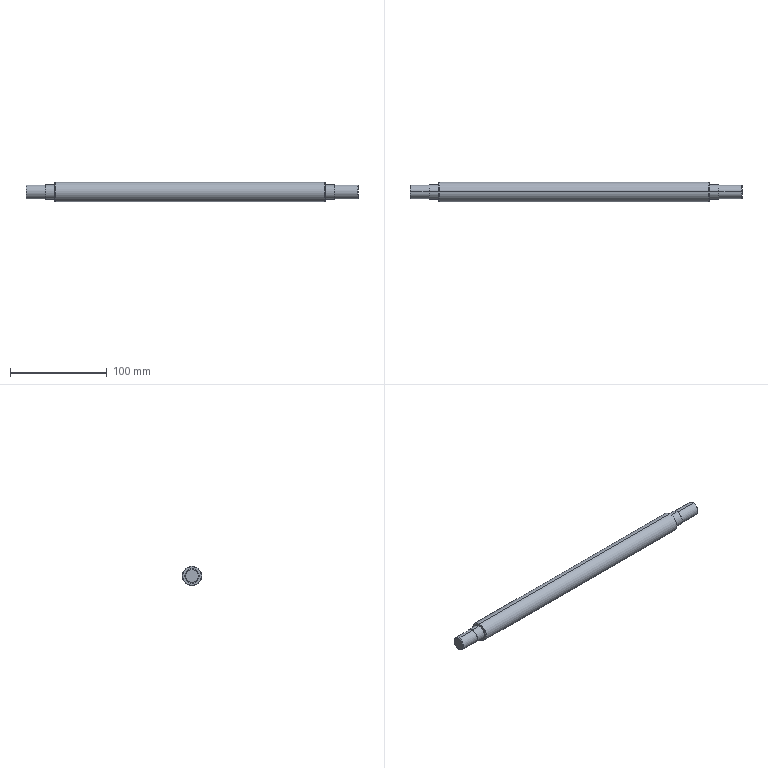Part | SolidWorks | features BaseBody 1 | 1 solid | 24 faces | box 344 x 20 x 20 mm | volume 98246 mm3 | cylinder 10 | cone 8 | plane 6 | commonest cylinder face diameters 14 x4 15 x4 20 x2
STEP:
#1=CARTESIAN_POINT('',(172.,0.,6.5));
#2=VERTEX_POINT('',#1);
#3=CARTESIAN_POINT('',(172.,0.,-6.5));
#4=VERTEX_POINT('',#3);
#5=CARTESIAN_POINT('',(172.,0.,0.));
#6=DIRECTION('',(-1.,0.,0.));
#7=DIRECTION('',(0.,0.,1.));
#8=AXIS2_PLACEMENT_3D('',#5,#6,#7);
#9=CIRCLE('',#8,6.5);
#10=EDGE_CURVE('',#2,#4,#9,.T.);
#11=ORIENTED_EDGE('',*,*,#10,.T.);
#12=CARTESIAN_POINT('',(171.5,0.,-7.));
#13=VERTEX_POINT('',#12);
#14=CARTESIAN_POINT('',(172.,0.,-6.5));
#15=DIRECTION('',(-0.7071,0.,-0.7071));
#16=VECTOR('',#15,1000.);
#17=LINE('',#14,#16);
#18=EDGE_CURVE('',#4,#13,#17,.T.);
#19=ORIENTED_EDGE('',*,*,#18,.T.);
#20=CARTESIAN_POINT('',(171.5,0.,7.));
#21=VERTEX_POINT('',#20);
#22=CARTESIAN_POINT('',(171.5,0.,0.));
#23=DIRECTION('',(-1.,0.,0.));
#24=DIRECTION('',(0.,0.,1.));
#25=AXIS2_PLACEMENT_3D('',#22,#23,#24);
#26=CIRCLE('',#25,7.);
#27=EDGE_CURVE('',#21,#13,#26,.T.);
#28=ORIENTED_EDGE('',*,*,#27,.F.);
#29=CARTESIAN_POINT('',(172.,0.,6.5));
#30=DIRECTION('',(-0.7071,0.,0.7071));
#31=VECTOR('',#30,1000.);
#32=LINE('',#29,#31);
#33=EDGE_CURVE('',#2,#21,#32,.T.);
#34=ORIENTED_EDGE('',*,*,#33,.F.);
#35=EDGE_LOOP('',(#11,#19,#28,#34));
#36=FACE_OUTER_BOUND('',#35,.T.);
#37=CARTESIAN_POINT('',(172.,0.,0.));
#38=DIRECTION('',(-1.,0.,0.));
#39=DIRECTION('',(0.,0.,1.));
#40=AXIS2_PLACEMENT_3D('',#37,#38,#39);
#41=CONICAL_SURFACE('',#40,6.5,0.7854);
#42=ADVANCED_FACE('',(#36),#41,.T.);
#43=ORIENTED_EDGE('',*,*,#27,.T.);
#44=CARTESIAN_POINT('',(148.,0.,-7.));
#45=VERTEX_POINT('',#44);
#46=CARTESIAN_POINT('',(-172.,0.,-7.));
#47=DIRECTION('',(-1.,0.,0.));
#48=VECTOR('',#47,1000.);
#49=LINE('',#46,#48);
#50=EDGE_CURVE('',#13,#45,#49,.T.);
#51=ORIENTED_EDGE('',*,*,#50,.T.);
#52=CARTESIAN_POINT('',(148.,0.,7.));
#53=VERTEX_POINT('',#52);
#54=CARTESIAN_POINT('',(148.,0.,0.));
#55=DIRECTION('',(-1.,0.,0.));
#56=DIRECTION('',(0.,0.,1.));
#57=AXIS2_PLACEMENT_3D('',#54,#55,#56);
#58=CIRCLE('',#57,7.);
#59=EDGE_CURVE('',#53,#45,#58,.T.);
#60=ORIENTED_EDGE('',*,*,#59,.F.);
#61=CARTESIAN_POINT('',(-172.,0.,7.));
#62=DIRECTION('',(-1.,0.,0.));
#63=VECTOR('',#62,1000.);
#64=LINE('',#61,#63);
#65=EDGE_CURVE('',#21,#53,#64,.T.);
#66=ORIENTED_EDGE('',*,*,#65,.F.);
#67=EDGE_LOOP('',(#43,#51,#60,#66));
#68=FACE_OUTER_BOUND('',#67,.T.);
#69=CARTESIAN_POINT('',(-172.,0.,0.));
#70=DIRECTION('',(-1.,0.,0.));
#71=DIRECTION('',(0.,0.,1.));
#72=AXIS2_PLACEMENT_3D('',#69,#70,#71);
#73=CYLINDRICAL_SURFACE('',#72,7.);
#74=ADVANCED_FACE('',(#68),#73,.T.);
#75=CARTESIAN_POINT('',(148.,0.,7.5));
#76=VERTEX_POINT('',#75);
#77=CARTESIAN_POINT('',(148.,0.,-7.5));
#78=VERTEX_POINT('',#77);
#79=CARTESIAN_POINT('',(148.,0.,0.));
#80=DIRECTION('',(-1.,0.,0.));
#81=DIRECTION('',(0.,0.,1.));
#82=AXIS2_PLACEMENT_3D('',#79,#80,#81);
#83=CIRCLE('',#82,7.5);
#84=EDGE_CURVE('',#76,#78,#83,.T.);
#85=ORIENTED_EDGE('',*,*,#84,.T.);
#86=CARTESIAN_POINT('',(138.,0.,-7.5));
#87=VERTEX_POINT('',#86);
#88=CARTESIAN_POINT('',(-172.,0.,-7.5));
#89=DIRECTION('',(-1.,0.,0.));
#90=VECTOR('',#89,1000.);
#91=LINE('',#88,#90);
#92=EDGE_CURVE('',#78,#87,#91,.T.);
#93=ORIENTED_EDGE('',*,*,#92,.T.);
#94=CARTESIAN_POINT('',(138.,0.,7.5));
#95=VERTEX_POINT('',#94);
#96=CARTESIAN_POINT('',(138.,0.,0.));
#97=DIRECTION('',(-1.,0.,0.));
#98=DIRECTION('',(0.,0.,1.));
#99=AXIS2_PLACEMENT_3D('',#96,#97,#98);
#100=CIRCLE('',#99,7.5);
#101=EDGE_CURVE('',#95,#87,#100,.T.);
#102=ORIENTED_EDGE('',*,*,#101,.F.);
#103=CARTESIAN_POINT('',(-172.,0.,7.5));
#104=DIRECTION('',(-1.,0.,0.));
#105=VECTOR('',#104,1000.);
#106=LINE('',#103,#105);
#107=EDGE_CURVE('',#76,#95,#106,.T.);
#108=ORIENTED_EDGE('',*,*,#107,.F.);
#109=EDGE_LOOP('',(#85,#93,#102,#108));
#110=FACE_OUTER_BOUND('',#109,.T.);
#111=CARTESIAN_POINT('',(-172.,0.,0.));
#112=DIRECTION('',(-1.,0.,0.));
#113=DIRECTION('',(0.,0.,1.));
#114=AXIS2_PLACEMENT_3D('',#111,#112,#113);
#115=CYLINDRICAL_SURFACE('',#114,7.5);
#116=ADVANCED_FACE('',(#110),#115,.T.);
#117=CARTESIAN_POINT('',(138.,0.,9.5));
#118=VERTEX_POINT('',#117);
#119=CARTESIAN_POINT('',(138.,0.,-9.5));
#120=VERTEX_POINT('',#119);
#121=CARTESIAN_POINT('',(138.,0.,0.));
#122=DIRECTION('',(-1.,0.,0.));
#123=DIRECTION('',(0.,0.,1.));
#124=AXIS2_PLACEMENT_3D('',#121,#122,#123);
#125=CIRCLE('',#124,9.5);
#126=EDGE_CURVE('',#118,#120,#125,.T.);
#127=ORIENTED_EDGE('',*,*,#126,.T.);
#128=CARTESIAN_POINT('',(137.5,0.,-10.));
#129=VERTEX_POINT('',#128);
#130=CARTESIAN_POINT('',(138.,0.,-9.5));
#131=DIRECTION('',(-0.7071,0.,-0.7071));
#132=VECTOR('',#131,1000.);
#133=LINE('',#130,#132);
#134=EDGE_CURVE('',#120,#129,#133,.T.);
#135=ORIENTED_EDGE('',*,*,#134,.T.);
#136=CARTESIAN_POINT('',(137.5,0.,10.));
#137=VERTEX_POINT('',#136);
#138=CARTESIAN_POINT('',(137.5,0.,0.));
#139=DIRECTION('',(-1.,0.,0.));
#140=DIRECTION('',(0.,0.,1.));
#141=AXIS2_PLACEMENT_3D('',#138,#139,#140);
#142=CIRCLE('',#141,10.);
#143=EDGE_CURVE('',#137,#129,#142,.T.);
#144=ORIENTED_EDGE('',*,*,#143,.F.);
#145=CARTESIAN_POINT('',(138.,0.,9.5));
#146=DIRECTION('',(-0.7071,0.,0.7071));
#147=VECTOR('',#146,1000.);
#148=LINE('',#145,#147);
#149=EDGE_CURVE('',#118,#137,#148,.T.);
#150=ORIENTED_EDGE('',*,*,#149,.F.);
#151=EDGE_LOOP('',(#127,#135,#144,#150));
#152=FACE_OUTER_BOUND('',#151,.T.);
#153=CARTESIAN_POINT('',(138.,0.,0.));
#154=DIRECTION('',(-1.,0.,0.));
#155=DIRECTION('',(0.,0.,1.));
#156=AXIS2_PLACEMENT_3D('',#153,#154,#155);
#157=CONICAL_SURFACE('',#156,9.5,0.7854);
#158=ADVANCED_FACE('',(#152),#157,.T.);
#159=ORIENTED_EDGE('',*,*,#143,.T.);
#160=CARTESIAN_POINT('',(-141.5,0.,-10.));
#161=VERTEX_POINT('',#160);
#162=CARTESIAN_POINT('',(-172.,0.,-10.));
#163=DIRECTION('',(-1.,0.,0.));
#164=VECTOR('',#163,1000.);
#165=LINE('',#162,#164);
#166=EDGE_CURVE('',#129,#161,#165,.T.);
#167=ORIENTED_EDGE('',*,*,#166,.T.);
#168=CARTESIAN_POINT('',(-141.5,0.,10.));
#169=VERTEX_POINT('',#168);
#170=CARTESIAN_POINT('',(-141.5,0.,0.));
#171=DIRECTION('',(-1.,0.,0.));
#172=DIRECTION('',(0.,0.,1.));
#173=AXIS2_PLACEMENT_3D('',#170,#171,#172);
#174=CIRCLE('',#173,10.);
#175=EDGE_CURVE('',#169,#161,#174,.T.);
#176=ORIENTED_EDGE('',*,*,#175,.F.);
#177=CARTESIAN_POINT('',(-172.,0.,10.));
#178=DIRECTION('',(-1.,0.,0.));
#179=VECTOR('',#178,1000.);
#180=LINE('',#177,#179);
#181=EDGE_CURVE('',#137,#169,#180,.T.);
#182=ORIENTED_EDGE('',*,*,#181,.F.);
#183=EDGE_LOOP('',(#159,#167,#176,#182));
#184=FACE_OUTER_BOUND('',#183,.T.);
#185=CARTESIAN_POINT('',(-172.,0.,0.));
#186=DIRECTION('',(-1.,0.,0.));
#187=DIRECTION('',(0.,0.,1.));
#188=AXIS2_PLACEMENT_3D('',#185,#186,#187);
#189=CYLINDRICAL_SURFACE('',#188,10.);
#190=ADVANCED_FACE('',(#184),#189,.T.);
#191=CARTESIAN_POINT('',(-142.,0.,9.5));
#192=VERTEX_POINT('',#191);
#193=CARTESIAN_POINT('',(-142.,0.,-9.5));
#194=VERTEX_POINT('',#193);
#195=CARTESIAN_POINT('',(-142.,0.,0.));
#196=DIRECTION('',(-1.,0.,0.));
#197=DIRECTION('',(0.,0.,1.));
#198=AXIS2_PLACEMENT_3D('',#195,#196,#197);
#199=CIRCLE('',#198,9.5);
#200=EDGE_CURVE('',#192,#194,#199,.T.);
#201=ORIENTED_EDGE('',*,*,#200,.F.);
#202=CARTESIAN_POINT('',(-141.5,0.,10.));
#203=DIRECTION('',(0.7071,0.,0.7071));
#204=VECTOR('',#203,1000.);
#205=LINE('',#202,#204);
#206=EDGE_CURVE('',#192,#169,#205,.T.);
#207=ORIENTED_EDGE('',*,*,#206,.T.);
#208=ORIENTED_EDGE('',*,*,#175,.T.);
#209=CARTESIAN_POINT('',(-141.5,0.,-10.));
#210=DIRECTION('',(0.7071,0.,-0.7071));
#211=VECTOR('',#210,1000.);
#212=LINE('',#209,#211);
#213=EDGE_CURVE('',#194,#161,#212,.T.);
#214=ORIENTED_EDGE('',*,*,#213,.F.);
#215=EDGE_LOOP('',(#201,#207,#208,#214));
#216=FACE_OUTER_BOUND('',#215,.T.);
#217=CARTESIAN_POINT('',(-141.5,0.,0.));
#218=DIRECTION('',(1.,0.,0.));
#219=DIRECTION('',(0.,0.,-1.));
#220=AXIS2_PLACEMENT_3D('',#217,#218,#219);
#221=CONICAL_SURFACE('',#220,10.,0.7854);
#222=ADVANCED_FACE('',(#216),#221,.T.);
#223=CARTESIAN_POINT('',(-142.,0.,7.5));
#224=VERTEX_POINT('',#223);
#225=CARTESIAN_POINT('',(-142.,0.,-7.5));
#226=VERTEX_POINT('',#225);
#227=CARTESIAN_POINT('',(-142.,0.,0.));
#228=DIRECTION('',(-1.,0.,0.));
#229=DIRECTION('',(0.,0.,1.));
#230=AXIS2_PLACEMENT_3D('',#227,#228,#229);
#231=CIRCLE('',#230,7.5);
#232=EDGE_CURVE('',#224,#226,#231,.T.);
#233=ORIENTED_EDGE('',*,*,#232,.T.);
#234=CARTESIAN_POINT('',(-152.,0.,-7.5));
#235=VERTEX_POINT('',#234);
#236=CARTESIAN_POINT('',(-172.,0.,-7.5));
#237=DIRECTION('',(-1.,0.,0.));
#238=VECTOR('',#237,1000.);
#239=LINE('',#236,#238);
#240=EDGE_CURVE('',#226,#235,#239,.T.);
#241=ORIENTED_EDGE('',*,*,#240,.T.);
#242=CARTESIAN_POINT('',(-152.,0.,7.5));
#243=VERTEX_POINT('',#242);
#244=CARTESIAN_POINT('',(-152.,0.,0.));
#245=DIRECTION('',(-1.,0.,0.));
#246=DIRECTION('',(0.,0.,1.));
#247=AXIS2_PLACEMENT_3D('',#244,#245,#246);
#248=CIRCLE('',#247,7.5);
#249=EDGE_CURVE('',#243,#235,#248,.T.);
#250=ORIENTED_EDGE('',*,*,#249,.F.);
#251=CARTESIAN_POINT('',(-172.,0.,7.5));
#252=DIRECTION('',(-1.,0.,0.));
#253=VECTOR('',#252,1000.);
#254=LINE('',#251,#253);
#255=EDGE_CURVE('',#224,#243,#254,.T.);
#256=ORIENTED_EDGE('',*,*,#255,.F.);
#257=EDGE_LOOP('',(#233,#241,#250,#256));
#258=FACE_OUTER_BOUND('',#257,.T.);
#259=CARTESIAN_POINT('',(-172.,0.,0.));
#260=DIRECTION('',(-1.,0.,0.));
#261=DIRECTION('',(0.,0.,1.));
#262=AXIS2_PLACEMENT_3D('',#259,#260,#261);
#263=CYLINDRICAL_SURFACE('',#262,7.5);
#264=ADVANCED_FACE('',(#258),#263,.T.);
#265=CARTESIAN_POINT('',(-152.,0.,7.));
#266=VERTEX_POINT('',#265);
#267=CARTESIAN_POINT('',(-152.,0.,-7.));
#268=VERTEX_POINT('',#267);
#269=CARTESIAN_POINT('',(-152.,0.,0.));
#270=DIRECTION('',(-1.,0.,0.));
#271=DIRECTION('',(0.,0.,1.));
#272=AXIS2_PLACEMENT_3D('',#269,#270,#271);
#273=CIRCLE('',#272,7.);
#274=EDGE_CURVE('',#266,#268,#273,.T.);
#275=ORIENTED_EDGE('',*,*,#274,.T.);
#276=CARTESIAN_POINT('',(-171.5,0.,-7.));
#277=VERTEX_POINT('',#276);
#278=CARTESIAN_POINT('',(-172.,0.,-7.));
#279=DIRECTION('',(-1.,0.,0.));
#280=VECTOR('',#279,1000.);
#281=LINE('',#278,#280);
#282=EDGE_CURVE('',#268,#277,#281,.T.);
#283=ORIENTED_EDGE('',*,*,#282,.T.);
#284=CARTESIAN_POINT('',(-171.5,0.,7.));
#285=VERTEX_POINT('',#284);
#286=CARTESIAN_POINT('',(-171.5,0.,0.));
#287=DIRECTION('',(-1.,0.,0.));
#288=DIRECTION('',(0.,0.,1.));
#289=AXIS2_PLACEMENT_3D('',#286,#287,#288);
#290=CIRCLE('',#289,7.);
#291=EDGE_CURVE('',#285,#277,#290,.T.);
#292=ORIENTED_EDGE('',*,*,#291,.F.);
#293=CARTESIAN_POINT('',(-172.,0.,7.));
#294=DIRECTION('',(-1.,0.,0.));
#295=VECTOR('',#294,1000.);
#296=LINE('',#293,#295);
#297=EDGE_CURVE('',#266,#285,#296,.T.);
#298=ORIENTED_EDGE('',*,*,#297,.F.);
#299=EDGE_LOOP('',(#275,#283,#292,#298));
#300=FACE_OUTER_BOUND('',#299,.T.);
#301=CARTESIAN_POINT('',(-172.,0.,0.));
#302=DIRECTION('',(-1.,0.,0.));
#303=DIRECTION('',(0.,0.,1.));
#304=AXIS2_PLACEMENT_3D('',#301,#302,#303);
#305=CYLINDRICAL_SURFACE('',#304,7.);
#306=ADVANCED_FACE('',(#300),#305,.T.);
#307=CARTESIAN_POINT('',(-172.,0.,6.5));
#308=VERTEX_POINT('',#307);
#309=CARTESIAN_POINT('',(-172.,0.,-6.5));
#310=VERTEX_POINT('',#309);
#311=CARTESIAN_POINT('',(-172.,0.,0.));
#312=DIRECTION('',(-1.,0.,0.));
#313=DIRECTION('',(0.,0.,1.));
#314=AXIS2_PLACEMENT_3D('',#311,#312,#313);
#315=CIRCLE('',#314,6.5);
#316=EDGE_CURVE('',#308,#310,#315,.T.);
#317=ORIENTED_EDGE('',*,*,#316,.F.);
#318=CARTESIAN_POINT('',(-171.5,0.,7.));
#319=DIRECTION('',(0.7071,0.,0.7071));
#320=VECTOR('',#319,1000.);
#321=LINE('',#318,#320);
#322=EDGE_CURVE('',#308,#285,#321,.T.);
#323=ORIENTED_EDGE('',*,*,#322,.T.);
#324=ORIENTED_EDGE('',*,*,#291,.T.);
#325=CARTESIAN_POINT('',(-171.5,0.,-7.));
#326=DIRECTION('',(0.7071,0.,-0.7071));
#327=VECTOR('',#326,1000.);
#328=LINE('',#325,#327);
#329=EDGE_CURVE('',#310,#277,#328,.T.);
#330=ORIENTED_EDGE('',*,*,#329,.F.);
#331=EDGE_LOOP('',(#317,#323,#324,#330));
#332=FACE_OUTER_BOUND('',#331,.T.);
#333=CARTESIAN_POINT('',(-171.5,0.,0.));
#334=DIRECTION('',(1.,0.,0.));
#335=DIRECTION('',(0.,0.,-1.));
#336=AXIS2_PLACEMENT_3D('',#333,#334,#335);
#337=CONICAL_SURFACE('',#336,7.,0.7854);
#338=ADVANCED_FACE('',(#332),#337,.T.);
#339=ORIENTED_EDGE('',*,*,#10,.F.);
#340=CARTESIAN_POINT('',(172.,0.,0.));
#341=DIRECTION('',(-1.,0.,0.));
#342=DIRECTION('',(0.,0.,1.));
#343=AXIS2_PLACEMENT_3D('',#340,#341,#342);
#344=CIRCLE('',#343,6.5);
#345=EDGE_CURVE('',#4,#2,#344,.T.);
#346=ORIENTED_EDGE('',*,*,#345,.F.);
#347=EDGE_LOOP('',(#339,#346));
#348=FACE_OUTER_BOUND('',#347,.T.);
#349=CARTESIAN_POINT('',(172.,6.5,0.));
#350=DIRECTION('',(-1.,0.,0.));
#351=DIRECTION('',(0.,0.,1.));
#352=AXIS2_PLACEMENT_3D('',#349,#350,#351);
#353=PLANE('',#352);
#354=ADVANCED_FACE('',(#348),#353,.F.);
#355=ORIENTED_EDGE('',*,*,#59,.T.);
#356=CARTESIAN_POINT('',(148.,0.,0.));
#357=DIRECTION('',(-1.,0.,0.));
#358=DIRECTION('',(0.,0.,1.));
#359=AXIS2_PLACEMENT_3D('',#356,#357,#358);
#360=CIRCLE('',#359,7.);
#361=EDGE_CURVE('',#45,#53,#360,.T.);
#362=ORIENTED_EDGE('',*,*,#361,.T.);
#363=EDGE_LOOP('',(#355,#362));
#364=FACE_BOUND('',#363,.T.);
#365=ORIENTED_EDGE('',*,*,#84,.F.);
#366=CARTESIAN_POINT('',(148.,0.,0.));
#367=DIRECTION('',(-1.,0.,0.));
#368=DIRECTION('',(0.,0.,1.));
#369=AXIS2_PLACEMENT_3D('',#366,#367,#368);
#370=CIRCLE('',#369,7.5);
#371=EDGE_CURVE('',#78,#76,#370,.T.);
#372=ORIENTED_EDGE('',*,*,#371,.F.);
#373=EDGE_LOOP('',(#365,#372));
#374=FACE_OUTER_BOUND('',#373,.T.);
#375=CARTESIAN_POINT('',(148.,7.5,0.));
#376=DIRECTION('',(-1.,0.,0.));
#377=DIRECTION('',(0.,0.,1.));
#378=AXIS2_PLACEMENT_3D('',#375,#376,#377);
#379=PLANE('',#378);
#380=ADVANCED_FACE('',(#364,#374),#379,.F.);
#381=ORIENTED_EDGE('',*,*,#101,.T.);
#382=CARTESIAN_POINT('',(138.,0.,0.));
#383=DIRECTION('',(-1.,0.,0.));
#384=DIRECTION('',(0.,0.,1.));
#385=AXIS2_PLACEMENT_3D('',#382,#383,#384);
#386=CIRCLE('',#385,7.5);
#387=EDGE_CURVE('',#87,#95,#386,.T.);
#388=ORIENTED_EDGE('',*,*,#387,.T.);
#389=EDGE_LOOP('',(#381,#388));
#390=FACE_BOUND('',#389,.T.);
#391=ORIENTED_EDGE('',*,*,#126,.F.);
#392=CARTESIAN_POINT('',(138.,0.,0.));
#393=DIRECTION('',(-1.,0.,0.));
#394=DIRECTION('',(0.,0.,1.));
#395=AXIS2_PLACEMENT_3D('',#392,#393,#394);
#396=CIRCLE('',#395,9.5);
#397=EDGE_CURVE('',#120,#118,#396,.T.);
#398=ORIENTED_EDGE('',*,*,#397,.F.);
#399=EDGE_LOOP('',(#391,#398));
#400=FACE_OUTER_BOUND('',#399,.T.);
#401=CARTESIAN_POINT('',(138.,9.5,0.));
#402=DIRECTION('',(-1.,0.,0.));
#403=DIRECTION('',(0.,0.,1.));
#404=AXIS2_PLACEMENT_3D('',#401,#402,#403);
#405=PLANE('',#404);
#406=ADVANCED_FACE('',(#390,#400),#405,.F.);
#407=ORIENTED_EDGE('',*,*,#232,.F.);
#408=CARTESIAN_POINT('',(-142.,0.,0.));
#409=DIRECTION('',(-1.,0.,0.));
#410=DIRECTION('',(0.,0.,1.));
#411=AXIS2_PLACEMENT_3D('',#408,#409,#410);
#412=CIRCLE('',#411,7.5);
#413=EDGE_CURVE('',#226,#224,#412,.T.);
#414=ORIENTED_EDGE('',*,*,#413,.F.);
#415=EDGE_LOOP('',(#407,#414));
#416=FACE_BOUND('',#415,.T.);
#417=CARTESIAN_POINT('',(-142.,0.,0.));
#418=DIRECTION('',(-1.,0.,0.));
#419=DIRECTION('',(0.,0.,1.));
#420=AXIS2_PLACEMENT_3D('',#417,#418,#419);
#421=CIRCLE('',#420,9.5);
#422=EDGE_CURVE('',#194,#192,#421,.T.);
#423=ORIENTED_EDGE('',*,*,#422,.T.);
#424=ORIENTED_EDGE('',*,*,#200,.T.);
#425=EDGE_LOOP('',(#423,#424));
#426=FACE_OUTER_BOUND('',#425,.T.);
#427=CARTESIAN_POINT('',(-142.,7.5,0.));
#428=DIRECTION('',(1.,0.,0.));
#429=DIRECTION('',(0.,1.,0.));
#430=AXIS2_PLACEMENT_3D('',#427,#428,#429);
#431=PLANE('',#430);
#432=ADVANCED_FACE('',(#416,#426),#431,.F.);
#433=ORIENTED_EDGE('',*,*,#274,.F.);
#434=CARTESIAN_POINT('',(-152.,0.,0.));
#435=DIRECTION('',(-1.,0.,0.));
#436=DIRECTION('',(0.,0.,1.));
#437=AXIS2_PLACEMENT_3D('',#434,#435,#436);
#438=CIRCLE('',#437,7.);
#439=EDGE_CURVE('',#268,#266,#438,.T.);
#440=ORIENTED_EDGE('',*,*,#439,.F.);
#441=EDGE_LOOP('',(#433,#440));
#442=FACE_BOUND('',#441,.T.);
#443=ORIENTED_EDGE('',*,*,#249,.T.);
#444=CARTESIAN_POINT('',(-152.,0.,0.));
#445=DIRECTION('',(-1.,0.,0.));
#446=DIRECTION('',(0.,0.,1.));
#447=AXIS2_PLACEMENT_3D('',#444,#445,#446);
#448=CIRCLE('',#447,7.5);
#449=EDGE_CURVE('',#235,#243,#448,.T.);
#450=ORIENTED_EDGE('',*,*,#449,.T.);
#451=EDGE_LOOP('',(#443,#450));
#452=FACE_OUTER_BOUND('',#451,.T.);
#453=CARTESIAN_POINT('',(-152.,7.,0.));
#454=DIRECTION('',(1.,0.,0.));
#455=DIRECTION('',(0.,1.,0.));
#456=AXIS2_PLACEMENT_3D('',#453,#454,#455);
#457=PLANE('',#456);
#458=ADVANCED_FACE('',(#442,#452),#457,.F.);
#459=CARTESIAN_POINT('',(-172.,0.,0.));
#460=DIRECTION('',(-1.,0.,0.));
#461=DIRECTION('',(0.,0.,1.));
#462=AXIS2_PLACEMENT_3D('',#459,#460,#461);
#463=CIRCLE('',#462,6.5);
#464=EDGE_CURVE('',#310,#308,#463,.T.);
#465=ORIENTED_EDGE('',*,*,#464,.T.);
#466=ORIENTED_EDGE('',*,*,#316,.T.);
#467=EDGE_LOOP('',(#465,#466));
#468=FACE_OUTER_BOUND('',#467,.T.);
#469=CARTESIAN_POINT('',(-172.,0.,0.));
#470=DIRECTION('',(1.,0.,0.));
#471=DIRECTION('',(0.,1.,0.));
#472=AXIS2_PLACEMENT_3D('',#469,#470,#471);
#473=PLANE('',#472);
#474=ADVANCED_FACE('',(#468),#473,.F.);
#475=ORIENTED_EDGE('',*,*,#322,.F.);
#476=ORIENTED_EDGE('',*,*,#464,.F.);
#477=ORIENTED_EDGE('',*,*,#329,.T.);
#478=CARTESIAN_POINT('',(-171.5,0.,0.));
#479=DIRECTION('',(-1.,0.,0.));
#480=DIRECTION('',(0.,0.,1.));
#481=AXIS2_PLACEMENT_3D('',#478,#479,#480);
#482=CIRCLE('',#481,7.);
#483=EDGE_CURVE('',#277,#285,#482,.T.);
#484=ORIENTED_EDGE('',*,*,#483,.T.);
#485=EDGE_LOOP('',(#475,#476,#477,#484));
#486=FACE_OUTER_BOUND('',#485,.T.);
#487=CARTESIAN_POINT('',(-171.5,0.,0.));
#488=DIRECTION('',(1.,0.,0.));
#489=DIRECTION('',(0.,0.,-1.));
#490=AXIS2_PLACEMENT_3D('',#487,#488,#489);
#491=CONICAL_SURFACE('',#490,7.,0.7854);
#492=ADVANCED_FACE('',(#486),#491,.T.);
#493=ORIENTED_EDGE('',*,*,#282,.F.);
#494=ORIENTED_EDGE('',*,*,#439,.T.);
#495=ORIENTED_EDGE('',*,*,#297,.T.);
#496=ORIENTED_EDGE('',*,*,#483,.F.);
#497=EDGE_LOOP('',(#493,#494,#495,#496));
#498=FACE_OUTER_BOUND('',#497,.T.);
#499=CARTESIAN_POINT('',(-172.,0.,0.));
#500=DIRECTION('',(-1.,0.,0.));
#501=DIRECTION('',(0.,0.,1.));
#502=AXIS2_PLACEMENT_3D('',#499,#500,#501);
#503=CYLINDRICAL_SURFACE('',#502,7.);
#504=ADVANCED_FACE('',(#498),#503,.T.);
#505=ORIENTED_EDGE('',*,*,#240,.F.);
#506=ORIENTED_EDGE('',*,*,#413,.T.);
#507=ORIENTED_EDGE('',*,*,#255,.T.);
#508=ORIENTED_EDGE('',*,*,#449,.F.);
#509=EDGE_LOOP('',(#505,#506,#507,#508));
#510=FACE_OUTER_BOUND('',#509,.T.);
#511=CARTESIAN_POINT('',(-172.,0.,0.));
#512=DIRECTION('',(-1.,0.,0.));
#513=DIRECTION('',(0.,0.,1.));
#514=AXIS2_PLACEMENT_3D('',#511,#512,#513);
#515=CYLINDRICAL_SURFACE('',#514,7.5);
#516=ADVANCED_FACE('',(#510),#515,.T.);
#517=ORIENTED_EDGE('',*,*,#206,.F.);
#518=ORIENTED_EDGE('',*,*,#422,.F.);
#519=ORIENTED_EDGE('',*,*,#213,.T.);
#520=CARTESIAN_POINT('',(-141.5,0.,0.));
#521=DIRECTION('',(-1.,0.,0.));
#522=DIRECTION('',(0.,0.,1.));
#523=AXIS2_PLACEMENT_3D('',#520,#521,#522);
#524=CIRCLE('',#523,10.);
#525=EDGE_CURVE('',#161,#169,#524,.T.);
#526=ORIENTED_EDGE('',*,*,#525,.T.);
#527=EDGE_LOOP('',(#517,#518,#519,#526));
#528=FACE_OUTER_BOUND('',#527,.T.);
#529=CARTESIAN_POINT('',(-141.5,0.,0.));
#530=DIRECTION('',(1.,0.,0.));
#531=DIRECTION('',(0.,0.,-1.));
#532=AXIS2_PLACEMENT_3D('',#529,#530,#531);
#533=CONICAL_SURFACE('',#532,10.,0.7854);
#534=ADVANCED_FACE('',(#528),#533,.T.);
#535=ORIENTED_EDGE('',*,*,#166,.F.);
#536=CARTESIAN_POINT('',(137.5,0.,0.));
#537=DIRECTION('',(-1.,0.,0.));
#538=DIRECTION('',(0.,0.,1.));
#539=AXIS2_PLACEMENT_3D('',#536,#537,#538);
#540=CIRCLE('',#539,10.);
#541=EDGE_CURVE('',#129,#137,#540,.T.);
#542=ORIENTED_EDGE('',*,*,#541,.T.);
#543=ORIENTED_EDGE('',*,*,#181,.T.);
#544=ORIENTED_EDGE('',*,*,#525,.F.);
#545=EDGE_LOOP('',(#535,#542,#543,#544));
#546=FACE_OUTER_BOUND('',#545,.T.);
#547=CARTESIAN_POINT('',(-172.,0.,0.));
#548=DIRECTION('',(-1.,0.,0.));
#549=DIRECTION('',(0.,0.,1.));
#550=AXIS2_PLACEMENT_3D('',#547,#548,#549);
#551=CYLINDRICAL_SURFACE('',#550,10.);
#552=ADVANCED_FACE('',(#546),#551,.T.);
#553=ORIENTED_EDGE('',*,*,#134,.F.);
#554=ORIENTED_EDGE('',*,*,#397,.T.);
#555=ORIENTED_EDGE('',*,*,#149,.T.);
#556=ORIENTED_EDGE('',*,*,#541,.F.);
#557=EDGE_LOOP('',(#553,#554,#555,#556));
#558=FACE_OUTER_BOUND('',#557,.T.);
#559=CARTESIAN_POINT('',(138.,0.,0.));
#560=DIRECTION('',(-1.,0.,0.));
#561=DIRECTION('',(0.,0.,1.));
#562=AXIS2_PLACEMENT_3D('',#559,#560,#561);
#563=CONICAL_SURFACE('',#562,9.5,0.7854);
#564=ADVANCED_FACE('',(#558),#563,.T.);
#565=ORIENTED_EDGE('',*,*,#92,.F.);
#566=ORIENTED_EDGE('',*,*,#371,.T.);
#567=ORIENTED_EDGE('',*,*,#107,.T.);
#568=ORIENTED_EDGE('',*,*,#387,.F.);
#569=EDGE_LOOP('',(#565,#566,#567,#568));
#570=FACE_OUTER_BOUND('',#569,.T.);
#571=CARTESIAN_POINT('',(-172.,0.,0.));
#572=DIRECTION('',(-1.,0.,0.));
#573=DIRECTION('',(0.,0.,1.));
#574=AXIS2_PLACEMENT_3D('',#571,#572,#573);
#575=CYLINDRICAL_SURFACE('',#574,7.5);
#576=ADVANCED_FACE('',(#570),#575,.T.);
#577=ORIENTED_EDGE('',*,*,#50,.F.);
#578=CARTESIAN_POINT('',(171.5,0.,0.));
#579=DIRECTION('',(-1.,0.,0.));
#580=DIRECTION('',(0.,0.,1.));
#581=AXIS2_PLACEMENT_3D('',#578,#579,#580);
#582=CIRCLE('',#581,7.);
#583=EDGE_CURVE('',#13,#21,#582,.T.);
#584=ORIENTED_EDGE('',*,*,#583,.T.);
#585=ORIENTED_EDGE('',*,*,#65,.T.);
#586=ORIENTED_EDGE('',*,*,#361,.F.);
#587=EDGE_LOOP('',(#577,#584,#585,#586));
#588=FACE_OUTER_BOUND('',#587,.T.);
#589=CARTESIAN_POINT('',(-172.,0.,0.));
#590=DIRECTION('',(-1.,0.,0.));
#591=DIRECTION('',(0.,0.,1.));
#592=AXIS2_PLACEMENT_3D('',#589,#590,#591);
#593=CYLINDRICAL_SURFACE('',#592,7.);
#594=ADVANCED_FACE('',(#588),#593,.T.);
#595=ORIENTED_EDGE('',*,*,#18,.F.);
#596=ORIENTED_EDGE('',*,*,#345,.T.);
#597=ORIENTED_EDGE('',*,*,#33,.T.);
#598=ORIENTED_EDGE('',*,*,#583,.F.);
#599=EDGE_LOOP('',(#595,#596,#597,#598));
#600=FACE_OUTER_BOUND('',#599,.T.);
#601=CARTESIAN_POINT('',(172.,0.,0.));
#602=DIRECTION('',(-1.,0.,0.));
#603=DIRECTION('',(0.,0.,1.));
#604=AXIS2_PLACEMENT_3D('',#601,#602,#603);
#605=CONICAL_SURFACE('',#604,6.5,0.7854);
#606=ADVANCED_FACE('',(#600),#605,.T.);
#607=CLOSED_SHELL('',(#42,#74,#116,#158,#190,#222,#264,#306,#338,#354,#380,#406,#432,#458,#474,#492,#504,#516,#534,#552,#564,#576,#594,#606));
#608=MANIFOLD_SOLID_BREP('',#607);
#609=CARTESIAN_POINT('',(0.,0.,0.));
#610=DIRECTION('',(0.,0.,1.));
#611=DIRECTION('',(1.,0.,0.));
#612=AXIS2_PLACEMENT_3D('',#609,#610,#611);
#613=(LENGTH_UNIT()NAMED_UNIT(*)SI_UNIT(.MILLI.,.METRE.));
#614=UNCERTAINTY_MEASURE_WITH_UNIT(LENGTH_MEASURE(0.00001),#613,'','');
#615=(NAMED_UNIT(*)PLANE_ANGLE_UNIT()SI_UNIT($,.RADIAN.));
#616=(NAMED_UNIT(*)SI_UNIT($,.STERADIAN.)SOLID_ANGLE_UNIT());
#617=(GEOMETRIC_REPRESENTATION_CONTEXT(3)GLOBAL_UNCERTAINTY_ASSIGNED_CONTEXT((#614))GLOBAL_UNIT_ASSIGNED_CONTEXT((#613,#615,#616))REPRESENTATION_CONTEXT('',''));
#618=ADVANCED_BREP_SHAPE_REPRESENTATION('',(#608,#612),#617);